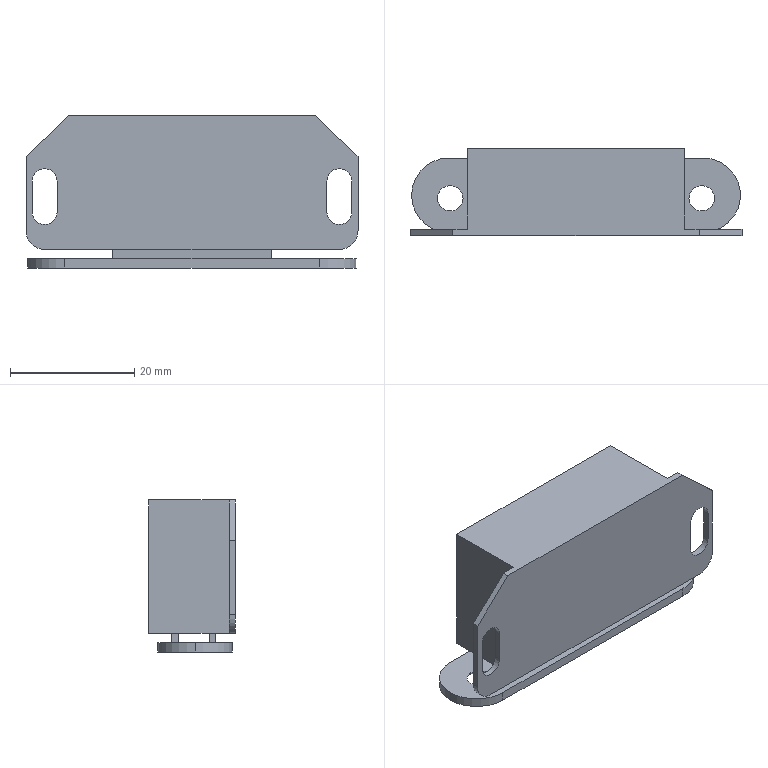Part | STEP file | AKB31 | 1 solid | 43 faces | box 53.5 x 14 x 24.5 mm | volume 11728 mm3 | plane 28 | cylinder 11 | cone 4 | commonest cylinder face diameters 4 x6 12 x3 6 x2